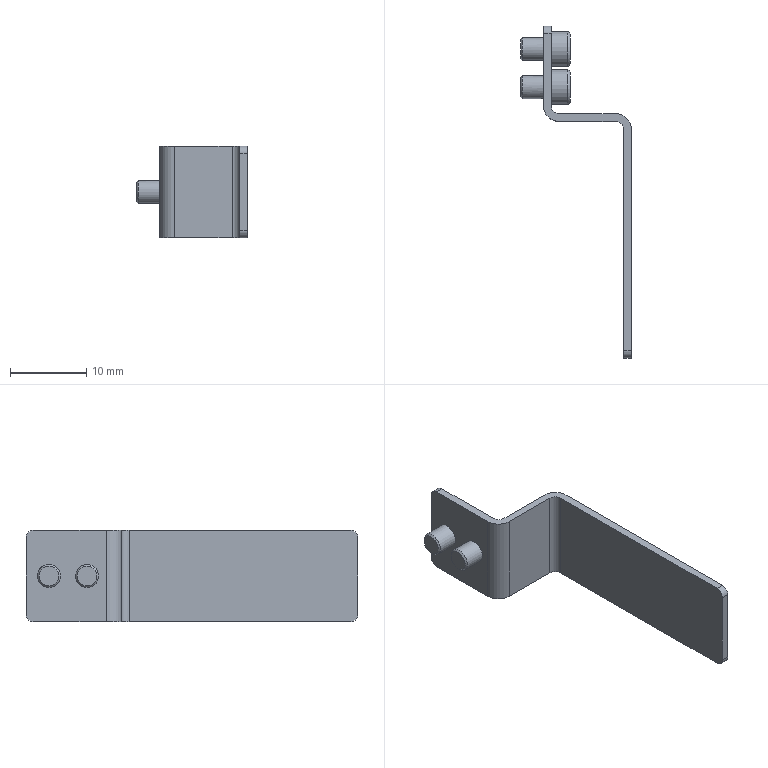Part | STEP file | BODY8_E-RAM6-S-640-ME30-C5 | 1 solid | 44 faces | box 14.5 x 43.5 x 12 mm | volume 744.799 mm3 | plane 28 | cylinder 12 | torus 2 | cone 2 | commonest cylinder face diameters 2 x6 3 x2 4 x2 4.5 x2
STEP:
#1=CARTESIAN_POINT('',(1.,3.,5.));
#2=VERTEX_POINT('',#1);
#3=CARTESIAN_POINT('',(1.,3.,-5.));
#4=VERTEX_POINT('',#3);
#5=CARTESIAN_POINT('',(1.,3.,6.));
#6=DIRECTION('',(0.,0.,-1.));
#7=VECTOR('',#6,1000.);
#8=LINE('',#5,#7);
#9=EDGE_CURVE('',#2,#4,#8,.T.);
#10=ORIENTED_EDGE('',*,*,#9,.T.);
#11=CARTESIAN_POINT('',(0.,3.,-5.));
#12=VERTEX_POINT('',#11);
#13=CARTESIAN_POINT('',(0.,3.,-5.));
#14=DIRECTION('',(-1.,0.,0.));
#15=VECTOR('',#14,1000.);
#16=LINE('',#13,#15);
#17=EDGE_CURVE('',#4,#12,#16,.T.);
#18=ORIENTED_EDGE('',*,*,#17,.T.);
#19=CARTESIAN_POINT('',(0.,3.,5.));
#20=VERTEX_POINT('',#19);
#21=CARTESIAN_POINT('',(0.,3.,6.));
#22=DIRECTION('',(0.,0.,-1.));
#23=VECTOR('',#22,1000.);
#24=LINE('',#21,#23);
#25=EDGE_CURVE('',#20,#12,#24,.T.);
#26=ORIENTED_EDGE('',*,*,#25,.F.);
#27=CARTESIAN_POINT('',(0.,3.,5.));
#28=DIRECTION('',(1.,0.,0.));
#29=VECTOR('',#28,1000.);
#30=LINE('',#27,#29);
#31=EDGE_CURVE('',#20,#2,#30,.T.);
#32=ORIENTED_EDGE('',*,*,#31,.T.);
#33=EDGE_LOOP('',(#10,#18,#26,#32));
#34=FACE_OUTER_BOUND('',#33,.T.);
#35=CARTESIAN_POINT('',(0.,3.,6.));
#36=DIRECTION('',(0.,-1.,0.));
#37=DIRECTION('',(0.,0.,-1.));
#38=AXIS2_PLACEMENT_3D('',#35,#36,#37);
#39=PLANE('',#38);
#40=ADVANCED_FACE('',(#34),#39,.F.);
#41=CARTESIAN_POINT('',(0.,2.,-6.));
#42=VERTEX_POINT('',#41);
#43=CARTESIAN_POINT('',(0.,-7.5,-6.));
#44=VERTEX_POINT('',#43);
#45=CARTESIAN_POINT('',(0.,3.,-6.));
#46=DIRECTION('',(0.,-1.,0.));
#47=VECTOR('',#46,1000.);
#48=LINE('',#45,#47);
#49=EDGE_CURVE('',#42,#44,#48,.T.);
#50=ORIENTED_EDGE('',*,*,#49,.T.);
#51=CARTESIAN_POINT('',(0.,-7.5,6.));
#52=VERTEX_POINT('',#51);
#53=CARTESIAN_POINT('',(0.,-7.5,6.));
#54=DIRECTION('',(0.,0.,1.));
#55=VECTOR('',#54,1000.);
#56=LINE('',#53,#55);
#57=EDGE_CURVE('',#44,#52,#56,.T.);
#58=ORIENTED_EDGE('',*,*,#57,.T.);
#59=CARTESIAN_POINT('',(0.,2.,6.));
#60=VERTEX_POINT('',#59);
#61=CARTESIAN_POINT('',(0.,3.,6.));
#62=DIRECTION('',(0.,-1.,0.));
#63=VECTOR('',#62,1000.);
#64=LINE('',#61,#63);
#65=EDGE_CURVE('',#60,#52,#64,.T.);
#66=ORIENTED_EDGE('',*,*,#65,.F.);
#67=CARTESIAN_POINT('',(0.,2.,5.));
#68=DIRECTION('',(-1.,0.,0.));
#69=DIRECTION('',(0.,0.,-1.));
#70=AXIS2_PLACEMENT_3D('',#67,#68,#69);
#71=CIRCLE('',#70,1.);
#72=EDGE_CURVE('',#60,#20,#71,.T.);
#73=ORIENTED_EDGE('',*,*,#72,.T.);
#74=ORIENTED_EDGE('',*,*,#25,.T.);
#75=CARTESIAN_POINT('',(0.,2.,-5.));
#76=DIRECTION('',(-1.,0.,0.));
#77=DIRECTION('',(0.,0.,-1.));
#78=AXIS2_PLACEMENT_3D('',#75,#76,#77);
#79=CIRCLE('',#78,1.);
#80=EDGE_CURVE('',#12,#42,#79,.T.);
#81=ORIENTED_EDGE('',*,*,#80,.T.);
#82=EDGE_LOOP('',(#50,#58,#66,#73,#74,#81));
#83=FACE_OUTER_BOUND('',#82,.T.);
#84=CARTESIAN_POINT('',(0.,-5.,-1.5));
#85=VERTEX_POINT('',#84);
#86=CARTESIAN_POINT('',(0.,-6.5,0.));
#87=VERTEX_POINT('',#86);
#88=CARTESIAN_POINT('',(0.,-5.,0.));
#89=DIRECTION('',(1.,0.,0.));
#90=DIRECTION('',(0.,0.,-1.));
#91=AXIS2_PLACEMENT_3D('',#88,#89,#90);
#92=CIRCLE('',#91,1.5);
#93=EDGE_CURVE('',#85,#87,#92,.T.);
#94=ORIENTED_EDGE('',*,*,#93,.T.);
#95=CARTESIAN_POINT('',(0.,-5.,0.));
#96=DIRECTION('',(1.,0.,0.));
#97=DIRECTION('',(0.,0.,-1.));
#98=AXIS2_PLACEMENT_3D('',#95,#96,#97);
#99=CIRCLE('',#98,1.5);
#100=EDGE_CURVE('',#87,#85,#99,.T.);
#101=ORIENTED_EDGE('',*,*,#100,.T.);
#102=EDGE_LOOP('',(#94,#101));
#103=FACE_BOUND('',#102,.T.);
#104=CARTESIAN_POINT('',(0.,0.,-1.5));
#105=VERTEX_POINT('',#104);
#106=CARTESIAN_POINT('',(0.,-1.5,0.));
#107=VERTEX_POINT('',#106);
#108=CARTESIAN_POINT('',(0.,0.,0.));
#109=DIRECTION('',(1.,0.,0.));
#110=DIRECTION('',(0.,0.,-1.));
#111=AXIS2_PLACEMENT_3D('',#108,#109,#110);
#112=CIRCLE('',#111,1.5);
#113=EDGE_CURVE('',#105,#107,#112,.T.);
#114=ORIENTED_EDGE('',*,*,#113,.T.);
#115=CARTESIAN_POINT('',(0.,0.,0.));
#116=DIRECTION('',(1.,0.,0.));
#117=DIRECTION('',(0.,0.,-1.));
#118=AXIS2_PLACEMENT_3D('',#115,#116,#117);
#119=CIRCLE('',#118,1.5);
#120=EDGE_CURVE('',#107,#105,#119,.T.);
#121=ORIENTED_EDGE('',*,*,#120,.T.);
#122=EDGE_LOOP('',(#114,#121));
#123=FACE_BOUND('',#122,.T.);
#124=CARTESIAN_POINT('',(0.,3.,6.));
#125=DIRECTION('',(1.,0.,0.));
#126=DIRECTION('',(0.,0.,-1.));
#127=AXIS2_PLACEMENT_3D('',#124,#125,#126);
#128=PLANE('',#127);
#129=ADVANCED_FACE('',(#83,#103,#123),#128,.F.);
#130=CARTESIAN_POINT('',(2.,-9.5,6.));
#131=VERTEX_POINT('',#130);
#132=CARTESIAN_POINT('',(9.5,-9.5,6.));
#133=VERTEX_POINT('',#132);
#134=CARTESIAN_POINT('',(0.,-9.5,6.));
#135=DIRECTION('',(1.,0.,0.));
#136=VECTOR('',#135,1000.);
#137=LINE('',#134,#136);
#138=EDGE_CURVE('',#131,#133,#137,.T.);
#139=ORIENTED_EDGE('',*,*,#138,.F.);
#140=CARTESIAN_POINT('',(2.,-9.5,-6.));
#141=VERTEX_POINT('',#140);
#142=CARTESIAN_POINT('',(2.,-9.5,6.));
#143=DIRECTION('',(0.,0.,-1.));
#144=VECTOR('',#143,1000.);
#145=LINE('',#142,#144);
#146=EDGE_CURVE('',#131,#141,#145,.T.);
#147=ORIENTED_EDGE('',*,*,#146,.T.);
#148=CARTESIAN_POINT('',(9.5,-9.5,-6.));
#149=VERTEX_POINT('',#148);
#150=CARTESIAN_POINT('',(0.,-9.5,-6.));
#151=DIRECTION('',(1.,0.,0.));
#152=VECTOR('',#151,1000.);
#153=LINE('',#150,#152);
#154=EDGE_CURVE('',#141,#149,#153,.T.);
#155=ORIENTED_EDGE('',*,*,#154,.T.);
#156=CARTESIAN_POINT('',(9.5,-9.5,6.));
#157=DIRECTION('',(0.,0.,1.));
#158=VECTOR('',#157,1000.);
#159=LINE('',#156,#158);
#160=EDGE_CURVE('',#149,#133,#159,.T.);
#161=ORIENTED_EDGE('',*,*,#160,.T.);
#162=EDGE_LOOP('',(#139,#147,#155,#161));
#163=FACE_OUTER_BOUND('',#162,.T.);
#164=CARTESIAN_POINT('',(0.,-9.5,6.));
#165=DIRECTION('',(0.,1.,0.));
#166=DIRECTION('',(0.,0.,1.));
#167=AXIS2_PLACEMENT_3D('',#164,#165,#166);
#168=PLANE('',#167);
#169=ADVANCED_FACE('',(#163),#168,.F.);
#170=CARTESIAN_POINT('',(10.5,-10.5,6.));
#171=VERTEX_POINT('',#170);
#172=CARTESIAN_POINT('',(10.5,-39.5,6.));
#173=VERTEX_POINT('',#172);
#174=CARTESIAN_POINT('',(10.5,-9.5,6.));
#175=DIRECTION('',(0.,-1.,0.));
#176=VECTOR('',#175,1000.);
#177=LINE('',#174,#176);
#178=EDGE_CURVE('',#171,#173,#177,.T.);
#179=ORIENTED_EDGE('',*,*,#178,.F.);
#180=CARTESIAN_POINT('',(10.5,-10.5,-6.));
#181=VERTEX_POINT('',#180);
#182=CARTESIAN_POINT('',(10.5,-10.5,-6.));
#183=DIRECTION('',(0.,0.,-1.));
#184=VECTOR('',#183,1000.);
#185=LINE('',#182,#184);
#186=EDGE_CURVE('',#171,#181,#185,.T.);
#187=ORIENTED_EDGE('',*,*,#186,.T.);
#188=CARTESIAN_POINT('',(10.5,-39.5,-6.));
#189=VERTEX_POINT('',#188);
#190=CARTESIAN_POINT('',(10.5,-9.5,-6.));
#191=DIRECTION('',(0.,-1.,0.));
#192=VECTOR('',#191,1000.);
#193=LINE('',#190,#192);
#194=EDGE_CURVE('',#181,#189,#193,.T.);
#195=ORIENTED_EDGE('',*,*,#194,.T.);
#196=CARTESIAN_POINT('',(10.5,-40.5,-5.));
#197=VERTEX_POINT('',#196);
#198=CARTESIAN_POINT('',(10.5,-39.5,-5.));
#199=DIRECTION('',(-1.,0.,0.));
#200=DIRECTION('',(0.,1.,0.));
#201=AXIS2_PLACEMENT_3D('',#198,#199,#200);
#202=CIRCLE('',#201,1.);
#203=EDGE_CURVE('',#189,#197,#202,.T.);
#204=ORIENTED_EDGE('',*,*,#203,.T.);
#205=CARTESIAN_POINT('',(10.5,-40.5,5.));
#206=VERTEX_POINT('',#205);
#207=CARTESIAN_POINT('',(10.5,-40.5,6.));
#208=DIRECTION('',(0.,0.,-1.));
#209=VECTOR('',#208,1000.);
#210=LINE('',#207,#209);
#211=EDGE_CURVE('',#206,#197,#210,.T.);
#212=ORIENTED_EDGE('',*,*,#211,.F.);
#213=CARTESIAN_POINT('',(10.5,-39.5,5.));
#214=DIRECTION('',(-1.,0.,0.));
#215=DIRECTION('',(0.,1.,0.));
#216=AXIS2_PLACEMENT_3D('',#213,#214,#215);
#217=CIRCLE('',#216,1.);
#218=EDGE_CURVE('',#206,#173,#217,.T.);
#219=ORIENTED_EDGE('',*,*,#218,.T.);
#220=EDGE_LOOP('',(#179,#187,#195,#204,#212,#219));
#221=FACE_OUTER_BOUND('',#220,.T.);
#222=CARTESIAN_POINT('',(10.5,-9.5,6.));
#223=DIRECTION('',(1.,0.,0.));
#224=DIRECTION('',(0.,1.,0.));
#225=AXIS2_PLACEMENT_3D('',#222,#223,#224);
#226=PLANE('',#225);
#227=ADVANCED_FACE('',(#221),#226,.F.);
#228=ORIENTED_EDGE('',*,*,#211,.T.);
#229=CARTESIAN_POINT('',(11.5,-40.5,-5.));
#230=VERTEX_POINT('',#229);
#231=CARTESIAN_POINT('',(11.5,-40.5,-5.));
#232=DIRECTION('',(1.,0.,0.));
#233=VECTOR('',#232,1000.);
#234=LINE('',#231,#233);
#235=EDGE_CURVE('',#197,#230,#234,.T.);
#236=ORIENTED_EDGE('',*,*,#235,.T.);
#237=CARTESIAN_POINT('',(11.5,-40.5,5.));
#238=VERTEX_POINT('',#237);
#239=CARTESIAN_POINT('',(11.5,-40.5,6.));
#240=DIRECTION('',(0.,0.,-1.));
#241=VECTOR('',#240,1000.);
#242=LINE('',#239,#241);
#243=EDGE_CURVE('',#238,#230,#242,.T.);
#244=ORIENTED_EDGE('',*,*,#243,.F.);
#245=CARTESIAN_POINT('',(10.5,-40.5,5.));
#246=DIRECTION('',(-1.,0.,0.));
#247=VECTOR('',#246,1000.);
#248=LINE('',#245,#247);
#249=EDGE_CURVE('',#238,#206,#248,.T.);
#250=ORIENTED_EDGE('',*,*,#249,.T.);
#251=EDGE_LOOP('',(#228,#236,#244,#250));
#252=FACE_OUTER_BOUND('',#251,.T.);
#253=CARTESIAN_POINT('',(10.5,-40.5,6.));
#254=DIRECTION('',(0.,1.,0.));
#255=DIRECTION('',(0.,0.,1.));
#256=AXIS2_PLACEMENT_3D('',#253,#254,#255);
#257=PLANE('',#256);
#258=ADVANCED_FACE('',(#252),#257,.F.);
#259=CARTESIAN_POINT('',(11.5,-39.5,-6.));
#260=VERTEX_POINT('',#259);
#261=CARTESIAN_POINT('',(11.5,-10.5,-6.));
#262=VERTEX_POINT('',#261);
#263=CARTESIAN_POINT('',(11.5,-8.5,-6.));
#264=DIRECTION('',(0.,1.,0.));
#265=VECTOR('',#264,1000.);
#266=LINE('',#263,#265);
#267=EDGE_CURVE('',#260,#262,#266,.T.);
#268=ORIENTED_EDGE('',*,*,#267,.T.);
#269=CARTESIAN_POINT('',(11.5,-10.5,6.));
#270=VERTEX_POINT('',#269);
#271=CARTESIAN_POINT('',(11.5,-10.5,6.));
#272=DIRECTION('',(0.,0.,1.));
#273=VECTOR('',#272,1000.);
#274=LINE('',#271,#273);
#275=EDGE_CURVE('',#262,#270,#274,.T.);
#276=ORIENTED_EDGE('',*,*,#275,.T.);
#277=CARTESIAN_POINT('',(11.5,-39.5,6.));
#278=VERTEX_POINT('',#277);
#279=CARTESIAN_POINT('',(11.5,-8.5,6.));
#280=DIRECTION('',(0.,1.,0.));
#281=VECTOR('',#280,1000.);
#282=LINE('',#279,#281);
#283=EDGE_CURVE('',#278,#270,#282,.T.);
#284=ORIENTED_EDGE('',*,*,#283,.F.);
#285=CARTESIAN_POINT('',(11.5,-39.5,5.));
#286=DIRECTION('',(1.,0.,0.));
#287=DIRECTION('',(0.,-1.,0.));
#288=AXIS2_PLACEMENT_3D('',#285,#286,#287);
#289=CIRCLE('',#288,1.);
#290=EDGE_CURVE('',#278,#238,#289,.T.);
#291=ORIENTED_EDGE('',*,*,#290,.T.);
#292=ORIENTED_EDGE('',*,*,#243,.T.);
#293=CARTESIAN_POINT('',(11.5,-39.5,-5.));
#294=DIRECTION('',(1.,0.,0.));
#295=DIRECTION('',(0.,-1.,0.));
#296=AXIS2_PLACEMENT_3D('',#293,#294,#295);
#297=CIRCLE('',#296,1.);
#298=EDGE_CURVE('',#230,#260,#297,.T.);
#299=ORIENTED_EDGE('',*,*,#298,.T.);
#300=EDGE_LOOP('',(#268,#276,#284,#291,#292,#299));
#301=FACE_OUTER_BOUND('',#300,.T.);
#302=CARTESIAN_POINT('',(11.5,-8.5,6.));
#303=DIRECTION('',(-1.,0.,0.));
#304=DIRECTION('',(0.,-1.,0.));
#305=AXIS2_PLACEMENT_3D('',#302,#303,#304);
#306=PLANE('',#305);
#307=ADVANCED_FACE('',(#301),#306,.F.);
#308=CARTESIAN_POINT('',(9.5,-8.5,6.));
#309=VERTEX_POINT('',#308);
#310=CARTESIAN_POINT('',(2.,-8.5,6.));
#311=VERTEX_POINT('',#310);
#312=CARTESIAN_POINT('',(1.,-8.5,6.));
#313=DIRECTION('',(-1.,0.,0.));
#314=VECTOR('',#313,1000.);
#315=LINE('',#312,#314);
#316=EDGE_CURVE('',#309,#311,#315,.T.);
#317=ORIENTED_EDGE('',*,*,#316,.F.);
#318=CARTESIAN_POINT('',(9.5,-8.5,-6.));
#319=VERTEX_POINT('',#318);
#320=CARTESIAN_POINT('',(9.5,-8.5,6.));
#321=DIRECTION('',(0.,0.,-1.));
#322=VECTOR('',#321,1000.);
#323=LINE('',#320,#322);
#324=EDGE_CURVE('',#309,#319,#323,.T.);
#325=ORIENTED_EDGE('',*,*,#324,.T.);
#326=CARTESIAN_POINT('',(2.,-8.5,-6.));
#327=VERTEX_POINT('',#326);
#328=CARTESIAN_POINT('',(1.,-8.5,-6.));
#329=DIRECTION('',(-1.,0.,0.));
#330=VECTOR('',#329,1000.);
#331=LINE('',#328,#330);
#332=EDGE_CURVE('',#319,#327,#331,.T.);
#333=ORIENTED_EDGE('',*,*,#332,.T.);
#334=CARTESIAN_POINT('',(2.,-8.5,6.));
#335=DIRECTION('',(0.,0.,1.));
#336=VECTOR('',#335,1000.);
#337=LINE('',#334,#336);
#338=EDGE_CURVE('',#327,#311,#337,.T.);
#339=ORIENTED_EDGE('',*,*,#338,.T.);
#340=EDGE_LOOP('',(#317,#325,#333,#339));
#341=FACE_OUTER_BOUND('',#340,.T.);
#342=CARTESIAN_POINT('',(1.,-8.5,6.));
#343=DIRECTION('',(0.,-1.,0.));
#344=DIRECTION('',(0.,0.,-1.));
#345=AXIS2_PLACEMENT_3D('',#342,#343,#344);
#346=PLANE('',#345);
#347=ADVANCED_FACE('',(#341),#346,.F.);
#348=CARTESIAN_POINT('',(1.,-7.5,6.));
#349=VERTEX_POINT('',#348);
#350=CARTESIAN_POINT('',(1.,2.,6.));
#351=VERTEX_POINT('',#350);
#352=CARTESIAN_POINT('',(1.,3.,6.));
#353=DIRECTION('',(0.,1.,0.));
#354=VECTOR('',#353,1000.);
#355=LINE('',#352,#354);
#356=EDGE_CURVE('',#349,#351,#355,.T.);
#357=ORIENTED_EDGE('',*,*,#356,.F.);
#358=CARTESIAN_POINT('',(1.,-7.5,-6.));
#359=VERTEX_POINT('',#358);
#360=CARTESIAN_POINT('',(1.,-7.5,-6.));
#361=DIRECTION('',(0.,0.,-1.));
#362=VECTOR('',#361,1000.);
#363=LINE('',#360,#362);
#364=EDGE_CURVE('',#349,#359,#363,.T.);
#365=ORIENTED_EDGE('',*,*,#364,.T.);
#366=CARTESIAN_POINT('',(1.,2.,-6.));
#367=VERTEX_POINT('',#366);
#368=CARTESIAN_POINT('',(1.,3.,-6.));
#369=DIRECTION('',(0.,1.,0.));
#370=VECTOR('',#369,1000.);
#371=LINE('',#368,#370);
#372=EDGE_CURVE('',#359,#367,#371,.T.);
#373=ORIENTED_EDGE('',*,*,#372,.T.);
#374=CARTESIAN_POINT('',(1.,2.,-5.));
#375=DIRECTION('',(1.,0.,0.));
#376=DIRECTION('',(0.,-1.,0.));
#377=AXIS2_PLACEMENT_3D('',#374,#375,#376);
#378=CIRCLE('',#377,1.);
#379=EDGE_CURVE('',#367,#4,#378,.T.);
#380=ORIENTED_EDGE('',*,*,#379,.T.);
#381=ORIENTED_EDGE('',*,*,#9,.F.);
#382=CARTESIAN_POINT('',(1.,2.,5.));
#383=DIRECTION('',(1.,0.,0.));
#384=DIRECTION('',(0.,-1.,0.));
#385=AXIS2_PLACEMENT_3D('',#382,#383,#384);
#386=CIRCLE('',#385,1.);
#387=EDGE_CURVE('',#2,#351,#386,.T.);
#388=ORIENTED_EDGE('',*,*,#387,.T.);
#389=EDGE_LOOP('',(#357,#365,#373,#380,#381,#388));
#390=FACE_OUTER_BOUND('',#389,.T.);
#391=CARTESIAN_POINT('',(1.,-7.25,0.));
#392=VERTEX_POINT('',#391);
#393=CARTESIAN_POINT('',(1.,-2.75,0.));
#394=VERTEX_POINT('',#393);
#395=CARTESIAN_POINT('',(1.,-5.,0.));
#396=DIRECTION('',(1.,0.,0.));
#397=DIRECTION('',(0.,-1.,0.));
#398=AXIS2_PLACEMENT_3D('',#395,#396,#397);
#399=CIRCLE('',#398,2.25);
#400=EDGE_CURVE('',#392,#394,#399,.T.);
#401=ORIENTED_EDGE('',*,*,#400,.F.);
#402=CARTESIAN_POINT('',(1.,-5.,0.));
#403=DIRECTION('',(1.,0.,0.));
#404=DIRECTION('',(0.,-1.,0.));
#405=AXIS2_PLACEMENT_3D('',#402,#403,#404);
#406=CIRCLE('',#405,2.25);
#407=EDGE_CURVE('',#394,#392,#406,.T.);
#408=ORIENTED_EDGE('',*,*,#407,.F.);
#409=EDGE_LOOP('',(#401,#408));
#410=FACE_BOUND('',#409,.T.);
#411=CARTESIAN_POINT('',(1.,-2.25,0.));
#412=VERTEX_POINT('',#411);
#413=CARTESIAN_POINT('',(1.,2.25,0.));
#414=VERTEX_POINT('',#413);
#415=CARTESIAN_POINT('',(1.,0.,0.));
#416=DIRECTION('',(1.,0.,0.));
#417=DIRECTION('',(0.,-1.,0.));
#418=AXIS2_PLACEMENT_3D('',#415,#416,#417);
#419=CIRCLE('',#418,2.25);
#420=EDGE_CURVE('',#412,#414,#419,.T.);
#421=ORIENTED_EDGE('',*,*,#420,.F.);
#422=CARTESIAN_POINT('',(1.,0.,0.));
#423=DIRECTION('',(1.,0.,0.));
#424=DIRECTION('',(0.,-1.,0.));
#425=AXIS2_PLACEMENT_3D('',#422,#423,#424);
#426=CIRCLE('',#425,2.25);
#427=EDGE_CURVE('',#414,#412,#426,.T.);
#428=ORIENTED_EDGE('',*,*,#427,.F.);
#429=EDGE_LOOP('',(#421,#428));
#430=FACE_BOUND('',#429,.T.);
#431=CARTESIAN_POINT('',(1.,3.,6.));
#432=DIRECTION('',(-1.,0.,0.));
#433=DIRECTION('',(0.,-1.,0.));
#434=AXIS2_PLACEMENT_3D('',#431,#432,#433);
#435=PLANE('',#434);
#436=ADVANCED_FACE('',(#390,#410,#430),#435,.F.);
#437=ORIENTED_EDGE('',*,*,#283,.T.);
#438=CARTESIAN_POINT('',(9.5,-10.5,6.));
#439=DIRECTION('',(0.,0.,1.));
#440=DIRECTION('',(-1.,0.,0.));
#441=AXIS2_PLACEMENT_3D('',#438,#439,#440);
#442=CIRCLE('',#441,2.);
#443=EDGE_CURVE('',#270,#309,#442,.T.);
#444=ORIENTED_EDGE('',*,*,#443,.T.);
#445=ORIENTED_EDGE('',*,*,#316,.T.);
#446=CARTESIAN_POINT('',(2.,-7.5,6.));
#447=DIRECTION('',(0.,0.,-1.));
#448=DIRECTION('',(-1.,0.,0.));
#449=AXIS2_PLACEMENT_3D('',#446,#447,#448);
#450=CIRCLE('',#449,1.);
#451=EDGE_CURVE('',#311,#349,#450,.T.);
#452=ORIENTED_EDGE('',*,*,#451,.T.);
#453=ORIENTED_EDGE('',*,*,#356,.T.);
#454=CARTESIAN_POINT('',(0.,2.,6.));
#455=DIRECTION('',(-1.,0.,0.));
#456=VECTOR('',#455,1000.);
#457=LINE('',#454,#456);
#458=EDGE_CURVE('',#351,#60,#457,.T.);
#459=ORIENTED_EDGE('',*,*,#458,.T.);
#460=ORIENTED_EDGE('',*,*,#65,.T.);
#461=CARTESIAN_POINT('',(2.,-7.5,6.));
#462=DIRECTION('',(0.,0.,1.));
#463=DIRECTION('',(-1.,0.,0.));
#464=AXIS2_PLACEMENT_3D('',#461,#462,#463);
#465=CIRCLE('',#464,2.);
#466=EDGE_CURVE('',#52,#131,#465,.T.);
#467=ORIENTED_EDGE('',*,*,#466,.T.);
#468=ORIENTED_EDGE('',*,*,#138,.T.);
#469=CARTESIAN_POINT('',(9.5,-10.5,6.));
#470=DIRECTION('',(0.,0.,-1.));
#471=DIRECTION('',(-1.,0.,0.));
#472=AXIS2_PLACEMENT_3D('',#469,#470,#471);
#473=CIRCLE('',#472,1.);
#474=EDGE_CURVE('',#133,#171,#473,.T.);
#475=ORIENTED_EDGE('',*,*,#474,.T.);
#476=ORIENTED_EDGE('',*,*,#178,.T.);
#477=CARTESIAN_POINT('',(0.,-39.5,6.));
#478=DIRECTION('',(1.,0.,0.));
#479=VECTOR('',#478,1000.);
#480=LINE('',#477,#479);
#481=EDGE_CURVE('',#173,#278,#480,.T.);
#482=ORIENTED_EDGE('',*,*,#481,.T.);
#483=EDGE_LOOP('',(#437,#444,#445,#452,#453,#459,#460,#467,#468,#475,#476,#482));
#484=FACE_OUTER_BOUND('',#483,.T.);
#485=CARTESIAN_POINT('',(0.,0.,6.));
#486=DIRECTION('',(0.,0.,-1.));
#487=DIRECTION('',(-1.,0.,0.));
#488=AXIS2_PLACEMENT_3D('',#485,#486,#487);
#489=PLANE('',#488);
#490=ADVANCED_FACE('',(#484),#489,.F.);
#491=ORIENTED_EDGE('',*,*,#332,.F.);
#492=CARTESIAN_POINT('',(9.5,-10.5,-6.));
#493=DIRECTION('',(0.,0.,-1.));
#494=DIRECTION('',(-1.,0.,0.));
#495=AXIS2_PLACEMENT_3D('',#492,#493,#494);
#496=CIRCLE('',#495,2.);
#497=EDGE_CURVE('',#319,#262,#496,.T.);
#498=ORIENTED_EDGE('',*,*,#497,.T.);
#499=ORIENTED_EDGE('',*,*,#267,.F.);
#500=CARTESIAN_POINT('',(10.5,-39.5,-6.));
#501=DIRECTION('',(-1.,0.,0.));
#502=VECTOR('',#501,1000.);
#503=LINE('',#500,#502);
#504=EDGE_CURVE('',#260,#189,#503,.T.);
#505=ORIENTED_EDGE('',*,*,#504,.T.);
#506=ORIENTED_EDGE('',*,*,#194,.F.);
#507=CARTESIAN_POINT('',(9.5,-10.5,-6.));
#508=DIRECTION('',(0.,0.,1.));
#509=DIRECTION('',(-1.,0.,0.));
#510=AXIS2_PLACEMENT_3D('',#507,#508,#509);
#511=CIRCLE('',#510,1.);
#512=EDGE_CURVE('',#181,#149,#511,.T.);
#513=ORIENTED_EDGE('',*,*,#512,.T.);
#514=ORIENTED_EDGE('',*,*,#154,.F.);
#515=CARTESIAN_POINT('',(2.,-7.5,-6.));
#516=DIRECTION('',(0.,0.,-1.));
#517=DIRECTION('',(-1.,0.,0.));
#518=AXIS2_PLACEMENT_3D('',#515,#516,#517);
#519=CIRCLE('',#518,2.);
#520=EDGE_CURVE('',#141,#44,#519,.T.);
#521=ORIENTED_EDGE('',*,*,#520,.T.);
#522=ORIENTED_EDGE('',*,*,#49,.F.);
#523=CARTESIAN_POINT('',(1.,2.,-6.));
#524=DIRECTION('',(1.,0.,0.));
#525=VECTOR('',#524,1000.);
#526=LINE('',#523,#525);
#527=EDGE_CURVE('',#42,#367,#526,.T.);
#528=ORIENTED_EDGE('',*,*,#527,.T.);
#529=ORIENTED_EDGE('',*,*,#372,.F.);
#530=CARTESIAN_POINT('',(2.,-7.5,-6.));
#531=DIRECTION('',(0.,0.,1.));
#532=DIRECTION('',(-1.,0.,0.));
#533=AXIS2_PLACEMENT_3D('',#530,#531,#532);
#534=CIRCLE('',#533,1.);
#535=EDGE_CURVE('',#359,#327,#534,.T.);
#536=ORIENTED_EDGE('',*,*,#535,.T.);
#537=EDGE_LOOP('',(#491,#498,#499,#505,#506,#513,#514,#521,#522,#528,#529,#536));
#538=FACE_OUTER_BOUND('',#537,.T.);
#539=CARTESIAN_POINT('',(0.,0.,-6.));
#540=DIRECTION('',(0.,0.,-1.));
#541=DIRECTION('',(-1.,0.,0.));
#542=AXIS2_PLACEMENT_3D('',#539,#540,#541);
#543=PLANE('',#542);
#544=ADVANCED_FACE('',(#538),#543,.T.);
#545=ORIENTED_EDGE('',*,*,#420,.T.);
#546=CARTESIAN_POINT('',(3.12,2.25,0.));
#547=VERTEX_POINT('',#546);
#548=CARTESIAN_POINT('',(3.5,2.25,0.));
#549=DIRECTION('',(1.,0.,0.));
#550=VECTOR('',#549,2.25);
#551=LINE('',#548,#550);
#552=EDGE_CURVE('',#414,#547,#551,.T.);
#553=ORIENTED_EDGE('',*,*,#552,.T.);
#554=CARTESIAN_POINT('',(3.12,-2.25,0.));
#555=VERTEX_POINT('',#554);
#556=CARTESIAN_POINT('',(3.12,0.,0.));
#557=DIRECTION('',(-1.,0.,0.));
#558=DIRECTION('',(0.,1.,0.));
#559=AXIS2_PLACEMENT_3D('',#556,#557,#558);
#560=CIRCLE('',#559,2.25);
#561=EDGE_CURVE('',#547,#555,#560,.T.);
#562=ORIENTED_EDGE('',*,*,#561,.T.);
#563=CARTESIAN_POINT('',(3.12,0.,0.));
#564=DIRECTION('',(-1.,0.,0.));
#565=DIRECTION('',(0.,1.,0.));
#566=AXIS2_PLACEMENT_3D('',#563,#564,#565);
#567=CIRCLE('',#566,2.25);
#568=EDGE_CURVE('',#555,#547,#567,.T.);
#569=ORIENTED_EDGE('',*,*,#568,.T.);
#570=ORIENTED_EDGE('',*,*,#552,.F.);
#571=ORIENTED_EDGE('',*,*,#427,.T.);
#572=EDGE_LOOP('',(#545,#553,#562,#569,#570,#571));
#573=FACE_OUTER_BOUND('',#572,.T.);
#574=CARTESIAN_POINT('',(3.5,0.,0.));
#575=DIRECTION('',(-1.,0.,0.));
#576=DIRECTION('',(0.,-1.,0.));
#577=AXIS2_PLACEMENT_3D('',#574,#575,#576);
#578=CYLINDRICAL_SURFACE('',#577,2.25);
#579=ADVANCED_FACE('',(#573),#578,.T.);
#580=CARTESIAN_POINT('',(3.5,1.87,0.));
#581=VERTEX_POINT('',#580);
#582=CARTESIAN_POINT('',(3.5,-1.87,0.));
#583=VERTEX_POINT('',#582);
#584=CARTESIAN_POINT('',(3.5,0.,0.));
#585=DIRECTION('',(1.,0.,0.));
#586=DIRECTION('',(0.,1.,0.));
#587=AXIS2_PLACEMENT_3D('',#584,#585,#586);
#588=CIRCLE('',#587,1.87);
#589=EDGE_CURVE('',#581,#583,#588,.T.);
#590=ORIENTED_EDGE('',*,*,#589,.T.);
#591=CARTESIAN_POINT('',(3.5,0.,0.));
#592=DIRECTION('',(1.,0.,0.));
#593=DIRECTION('',(0.,1.,0.));
#594=AXIS2_PLACEMENT_3D('',#591,#592,#593);
#595=CIRCLE('',#594,1.87);
#596=EDGE_CURVE('',#583,#581,#595,.T.);
#597=ORIENTED_EDGE('',*,*,#596,.T.);
#598=EDGE_LOOP('',(#590,#597));
#599=FACE_OUTER_BOUND('',#598,.T.);
#600=CARTESIAN_POINT('',(3.5,0.5774,-1.));
#601=VERTEX_POINT('',#600);
#602=CARTESIAN_POINT('',(3.5,1.155,0.));
#603=VERTEX_POINT('',#602);
#604=CARTESIAN_POINT('',(3.5,0.5774,-1.));
#605=DIRECTION('',(0.,0.5,0.866));
#606=VECTOR('',#605,1000.);
#607=LINE('',#604,#606);
#608=EDGE_CURVE('',#601,#603,#607,.T.);
#609=ORIENTED_EDGE('',*,*,#608,.F.);
#610=CARTESIAN_POINT('',(3.5,-0.5774,-1.));
#611=VERTEX_POINT('',#610);
#612=CARTESIAN_POINT('',(3.5,-0.5774,-1.));
#613=DIRECTION('',(0.,1.,0.));
#614=VECTOR('',#613,1000.);
#615=LINE('',#612,#614);
#616=EDGE_CURVE('',#611,#601,#615,.T.);
#617=ORIENTED_EDGE('',*,*,#616,.F.);
#618=CARTESIAN_POINT('',(3.5,-1.155,0.));
#619=VERTEX_POINT('',#618);
#620=CARTESIAN_POINT('',(3.5,-1.155,0.));
#621=DIRECTION('',(0.,0.5,-0.866));
#622=VECTOR('',#621,1000.);
#623=LINE('',#620,#622);
#624=EDGE_CURVE('',#619,#611,#623,.T.);
#625=ORIENTED_EDGE('',*,*,#624,.F.);
#626=CARTESIAN_POINT('',(3.5,-0.5774,1.));
#627=VERTEX_POINT('',#626);
#628=CARTESIAN_POINT('',(3.5,-0.5774,1.));
#629=DIRECTION('',(0.,-0.5,-0.866));
#630=VECTOR('',#629,1000.);
#631=LINE('',#628,#630);
#632=EDGE_CURVE('',#627,#619,#631,.T.);
#633=ORIENTED_EDGE('',*,*,#632,.F.);
#634=CARTESIAN_POINT('',(3.5,0.5774,1.));
#635=VERTEX_POINT('',#634);
#636=CARTESIAN_POINT('',(3.5,0.5774,1.));
#637=DIRECTION('',(0.,-1.,0.));
#638=VECTOR('',#637,1000.);
#639=LINE('',#636,#638);
#640=EDGE_CURVE('',#635,#627,#639,.T.);
#641=ORIENTED_EDGE('',*,*,#640,.F.);
#642=CARTESIAN_POINT('',(3.5,1.155,0.));
#643=DIRECTION('',(0.,-0.5,0.866));
#644=VECTOR('',#643,1000.);
#645=LINE('',#642,#644);
#646=EDGE_CURVE('',#603,#635,#645,.T.);
#647=ORIENTED_EDGE('',*,*,#646,.F.);
#648=EDGE_LOOP('',(#609,#617,#625,#633,#641,#647));
#649=FACE_BOUND('',#648,.T.);
#650=CARTESIAN_POINT('',(3.5,0.,0.));
#651=DIRECTION('',(1.,0.,0.));
#652=DIRECTION('',(0.,1.,0.));
#653=AXIS2_PLACEMENT_3D('',#650,#651,#652);
#654=PLANE('',#653);
#655=ADVANCED_FACE('',(#599,#649),#654,.T.);
#656=ORIENTED_EDGE('',*,*,#400,.T.);
#657=CARTESIAN_POINT('',(3.12,-2.75,0.));
#658=VERTEX_POINT('',#657);
#659=CARTESIAN_POINT('',(3.5,-2.75,0.));
#660=DIRECTION('',(1.,0.,0.));
#661=VECTOR('',#660,2.25);
#662=LINE('',#659,#661);
#663=EDGE_CURVE('',#394,#658,#662,.T.);
#664=ORIENTED_EDGE('',*,*,#663,.T.);
#665=CARTESIAN_POINT('',(3.12,-7.25,0.));
#666=VERTEX_POINT('',#665);
#667=CARTESIAN_POINT('',(3.12,-5.,0.));
#668=DIRECTION('',(-1.,0.,0.));
#669=DIRECTION('',(0.,1.,0.));
#670=AXIS2_PLACEMENT_3D('',#667,#668,#669);
#671=CIRCLE('',#670,2.25);
#672=EDGE_CURVE('',#658,#666,#671,.T.);
#673=ORIENTED_EDGE('',*,*,#672,.T.);
#674=CARTESIAN_POINT('',(3.12,-5.,0.));
#675=DIRECTION('',(-1.,0.,0.));
#676=DIRECTION('',(0.,1.,0.));
#677=AXIS2_PLACEMENT_3D('',#674,#675,#676);
#678=CIRCLE('',#677,2.25);
#679=EDGE_CURVE('',#666,#658,#678,.T.);
#680=ORIENTED_EDGE('',*,*,#679,.T.);
#681=ORIENTED_EDGE('',*,*,#663,.F.);
#682=ORIENTED_EDGE('',*,*,#407,.T.);
#683=EDGE_LOOP('',(#656,#664,#673,#680,#681,#682));
#684=FACE_OUTER_BOUND('',#683,.T.);
#685=CARTESIAN_POINT('',(3.5,-5.,0.));
#686=DIRECTION('',(-1.,0.,0.));
#687=DIRECTION('',(0.,-1.,0.));
#688=AXIS2_PLACEMENT_3D('',#685,#686,#687);
#689=CYLINDRICAL_SURFACE('',#688,2.25);
#690=ADVANCED_FACE('',(#684),#689,.T.);
#691=CARTESIAN_POINT('',(3.5,-3.13,0.));
#692=VERTEX_POINT('',#691);
#693=CARTESIAN_POINT('',(3.5,-6.87,0.));
#694=VERTEX_POINT('',#693);
#695=CARTESIAN_POINT('',(3.5,-5.,0.));
#696=DIRECTION('',(1.,0.,0.));
#697=DIRECTION('',(0.,1.,0.));
#698=AXIS2_PLACEMENT_3D('',#695,#696,#697);
#699=CIRCLE('',#698,1.87);
#700=EDGE_CURVE('',#692,#694,#699,.T.);
#701=ORIENTED_EDGE('',*,*,#700,.T.);
#702=CARTESIAN_POINT('',(3.5,-5.,0.));
#703=DIRECTION('',(1.,0.,0.));
#704=DIRECTION('',(0.,1.,0.));
#705=AXIS2_PLACEMENT_3D('',#702,#703,#704);
#706=CIRCLE('',#705,1.87);
#707=EDGE_CURVE('',#694,#692,#706,.T.);
#708=ORIENTED_EDGE('',*,*,#707,.T.);
#709=EDGE_LOOP('',(#701,#708));
#710=FACE_OUTER_BOUND('',#709,.T.);
#711=CARTESIAN_POINT('',(3.5,-4.423,-1.));
#712=VERTEX_POINT('',#711);
#713=CARTESIAN_POINT('',(3.5,-3.845,0.));
#714=VERTEX_POINT('',#713);
#715=CARTESIAN_POINT('',(3.5,-4.423,-1.));
#716=DIRECTION('',(0.,0.5,0.866));
#717=VECTOR('',#716,1000.);
#718=LINE('',#715,#717);
#719=EDGE_CURVE('',#712,#714,#718,.T.);
#720=ORIENTED_EDGE('',*,*,#719,.F.);
#721=CARTESIAN_POINT('',(3.5,-5.577,-1.));
#722=VERTEX_POINT('',#721);
#723=CARTESIAN_POINT('',(3.5,-5.577,-1.));
#724=DIRECTION('',(0.,1.,0.));
#725=VECTOR('',#724,1000.);
#726=LINE('',#723,#725);
#727=EDGE_CURVE('',#722,#712,#726,.T.);
#728=ORIENTED_EDGE('',*,*,#727,.F.);
#729=CARTESIAN_POINT('',(3.5,-6.155,0.));
#730=VERTEX_POINT('',#729);
#731=CARTESIAN_POINT('',(3.5,-6.155,0.));
#732=DIRECTION('',(0.,0.5,-0.866));
#733=VECTOR('',#732,1000.);
#734=LINE('',#731,#733);
#735=EDGE_CURVE('',#730,#722,#734,.T.);
#736=ORIENTED_EDGE('',*,*,#735,.F.);
#737=CARTESIAN_POINT('',(3.5,-5.577,1.));
#738=VERTEX_POINT('',#737);
#739=CARTESIAN_POINT('',(3.5,-5.577,1.));
#740=DIRECTION('',(0.,-0.5,-0.866));
#741=VECTOR('',#740,1000.);
#742=LINE('',#739,#741);
#743=EDGE_CURVE('',#738,#730,#742,.T.);
#744=ORIENTED_EDGE('',*,*,#743,.F.);
#745=CARTESIAN_POINT('',(3.5,-4.423,1.));
#746=VERTEX_POINT('',#745);
#747=CARTESIAN_POINT('',(3.5,-4.423,1.));
#748=DIRECTION('',(0.,-1.,0.));
#749=VECTOR('',#748,1000.);
#750=LINE('',#747,#749);
#751=EDGE_CURVE('',#746,#738,#750,.T.);
#752=ORIENTED_EDGE('',*,*,#751,.F.);
#753=CARTESIAN_POINT('',(3.5,-3.845,0.));
#754=DIRECTION('',(0.,-0.5,0.866));
#755=VECTOR('',#754,1000.);
#756=LINE('',#753,#755);
#757=EDGE_CURVE('',#714,#746,#756,.T.);
#758=ORIENTED_EDGE('',*,*,#757,.F.);
#759=EDGE_LOOP('',(#720,#728,#736,#744,#752,#758));
#760=FACE_BOUND('',#759,.T.);
#761=CARTESIAN_POINT('',(3.5,-5.,0.));
#762=DIRECTION('',(1.,0.,0.));
#763=DIRECTION('',(0.,1.,0.));
#764=AXIS2_PLACEMENT_3D('',#761,#762,#763);
#765=PLANE('',#764);
#766=ADVANCED_FACE('',(#710,#760),#765,.T.);
#767=ORIENTED_EDGE('',*,*,#608,.T.);
#768=CARTESIAN_POINT('',(2.4,1.155,0.));
#769=VERTEX_POINT('',#768);
#770=CARTESIAN_POINT('',(2.4,1.155,0.));
#771=DIRECTION('',(1.,0.,0.));
#772=VECTOR('',#771,1000.);
#773=LINE('',#770,#772);
#774=EDGE_CURVE('',#769,#603,#773,.T.);
#775=ORIENTED_EDGE('',*,*,#774,.F.);
#776=CARTESIAN_POINT('',(2.4,0.5774,-1.));
#777=VERTEX_POINT('',#776);
#778=CARTESIAN_POINT('',(2.4,0.5774,-1.));
#779=DIRECTION('',(0.,0.5,0.866));
#780=VECTOR('',#779,1000.);
#781=LINE('',#778,#780);
#782=EDGE_CURVE('',#777,#769,#781,.T.);
#783=ORIENTED_EDGE('',*,*,#782,.F.);
#784=CARTESIAN_POINT('',(2.4,0.5774,-1.));
#785=DIRECTION('',(1.,0.,0.));
#786=VECTOR('',#785,1000.);
#787=LINE('',#784,#786);
#788=EDGE_CURVE('',#777,#601,#787,.T.);
#789=ORIENTED_EDGE('',*,*,#788,.T.);
#790=EDGE_LOOP('',(#767,#775,#783,#789));
#791=FACE_OUTER_BOUND('',#790,.T.);
#792=CARTESIAN_POINT('',(2.4,0.5774,-1.));
#793=DIRECTION('',(0.,0.866,-0.5));
#794=DIRECTION('',(0.,0.5,0.866));
#795=AXIS2_PLACEMENT_3D('',#792,#793,#794);
#796=PLANE('',#795);
#797=ADVANCED_FACE('',(#791),#796,.F.);
#798=ORIENTED_EDGE('',*,*,#616,.T.);
#799=ORIENTED_EDGE('',*,*,#788,.F.);
#800=CARTESIAN_POINT('',(2.4,-0.5774,-1.));
#801=VERTEX_POINT('',#800);
#802=CARTESIAN_POINT('',(2.4,-0.5774,-1.));
#803=DIRECTION('',(0.,1.,0.));
#804=VECTOR('',#803,1000.);
#805=LINE('',#802,#804);
#806=EDGE_CURVE('',#801,#777,#805,.T.);
#807=ORIENTED_EDGE('',*,*,#806,.F.);
#808=CARTESIAN_POINT('',(2.4,-0.5774,-1.));
#809=DIRECTION('',(1.,0.,0.));
#810=VECTOR('',#809,1000.);
#811=LINE('',#808,#810);
#812=EDGE_CURVE('',#801,#611,#811,.T.);
#813=ORIENTED_EDGE('',*,*,#812,.T.);
#814=EDGE_LOOP('',(#798,#799,#807,#813));
#815=FACE_OUTER_BOUND('',#814,.T.);
#816=CARTESIAN_POINT('',(2.4,-0.5774,-1.));
#817=DIRECTION('',(0.,0.,-1.));
#818=DIRECTION('',(0.,1.,0.));
#819=AXIS2_PLACEMENT_3D('',#816,#817,#818);
#820=PLANE('',#819);
#821=ADVANCED_FACE('',(#815),#820,.F.);
#822=ORIENTED_EDGE('',*,*,#624,.T.);
#823=ORIENTED_EDGE('',*,*,#812,.F.);
#824=CARTESIAN_POINT('',(2.4,-1.155,0.));
#825=VERTEX_POINT('',#824);
#826=CARTESIAN_POINT('',(2.4,-1.155,0.));
#827=DIRECTION('',(0.,0.5,-0.866));
#828=VECTOR('',#827,1000.);
#829=LINE('',#826,#828);
#830=EDGE_CURVE('',#825,#801,#829,.T.);
#831=ORIENTED_EDGE('',*,*,#830,.F.);
#832=CARTESIAN_POINT('',(2.4,-1.155,0.));
#833=DIRECTION('',(1.,0.,0.));
#834=VECTOR('',#833,1000.);
#835=LINE('',#832,#834);
#836=EDGE_CURVE('',#825,#619,#835,.T.);
#837=ORIENTED_EDGE('',*,*,#836,.T.);
#838=EDGE_LOOP('',(#822,#823,#831,#837));
#839=FACE_OUTER_BOUND('',#838,.T.);
#840=CARTESIAN_POINT('',(2.4,-1.155,0.));
#841=DIRECTION('',(0.,-0.866,-0.5));
#842=DIRECTION('',(0.,0.5,-0.866));
#843=AXIS2_PLACEMENT_3D('',#840,#841,#842);
#844=PLANE('',#843);
#845=ADVANCED_FACE('',(#839),#844,.F.);
#846=ORIENTED_EDGE('',*,*,#632,.T.);
#847=ORIENTED_EDGE('',*,*,#836,.F.);
#848=CARTESIAN_POINT('',(2.4,-0.5774,1.));
#849=VERTEX_POINT('',#848);
#850=CARTESIAN_POINT('',(2.4,-0.5774,1.));
#851=DIRECTION('',(0.,-0.5,-0.866));
#852=VECTOR('',#851,1000.);
#853=LINE('',#850,#852);
#854=EDGE_CURVE('',#849,#825,#853,.T.);
#855=ORIENTED_EDGE('',*,*,#854,.F.);
#856=CARTESIAN_POINT('',(2.4,-0.5774,1.));
#857=DIRECTION('',(1.,0.,0.));
#858=VECTOR('',#857,1000.);
#859=LINE('',#856,#858);
#860=EDGE_CURVE('',#849,#627,#859,.T.);
#861=ORIENTED_EDGE('',*,*,#860,.T.);
#862=EDGE_LOOP('',(#846,#847,#855,#861));
#863=FACE_OUTER_BOUND('',#862,.T.);
#864=CARTESIAN_POINT('',(2.4,-0.5774,1.));
#865=DIRECTION('',(0.,-0.866,0.5));
#866=DIRECTION('',(0.,-0.5,-0.866));
#867=AXIS2_PLACEMENT_3D('',#864,#865,#866);
#868=PLANE('',#867);
#869=ADVANCED_FACE('',(#863),#868,.F.);
#870=ORIENTED_EDGE('',*,*,#640,.T.);
#871=ORIENTED_EDGE('',*,*,#860,.F.);
#872=CARTESIAN_POINT('',(2.4,0.5774,1.));
#873=VERTEX_POINT('',#872);
#874=CARTESIAN_POINT('',(2.4,0.5774,1.));
#875=DIRECTION('',(0.,-1.,0.));
#876=VECTOR('',#875,1000.);
#877=LINE('',#874,#876);
#878=EDGE_CURVE('',#873,#849,#877,.T.);
#879=ORIENTED_EDGE('',*,*,#878,.F.);
#880=CARTESIAN_POINT('',(2.4,0.5774,1.));
#881=DIRECTION('',(1.,0.,0.));
#882=VECTOR('',#881,1000.);
#883=LINE('',#880,#882);
#884=EDGE_CURVE('',#873,#635,#883,.T.);
#885=ORIENTED_EDGE('',*,*,#884,.T.);
#886=EDGE_LOOP('',(#870,#871,#879,#885));
#887=FACE_OUTER_BOUND('',#886,.T.);
#888=CARTESIAN_POINT('',(2.4,0.5774,1.));
#889=DIRECTION('',(0.,0.,1.));
#890=DIRECTION('',(1.,0.,0.));
#891=AXIS2_PLACEMENT_3D('',#888,#889,#890);
#892=PLANE('',#891);
#893=ADVANCED_FACE('',(#887),#892,.F.);
#894=ORIENTED_EDGE('',*,*,#646,.T.);
#895=ORIENTED_EDGE('',*,*,#884,.F.);
#896=CARTESIAN_POINT('',(2.4,1.155,0.));
#897=DIRECTION('',(0.,-0.5,0.866));
#898=VECTOR('',#897,1000.);
#899=LINE('',#896,#898);
#900=EDGE_CURVE('',#769,#873,#899,.T.);
#901=ORIENTED_EDGE('',*,*,#900,.F.);
#902=ORIENTED_EDGE('',*,*,#774,.T.);
#903=EDGE_LOOP('',(#894,#895,#901,#902));
#904=FACE_OUTER_BOUND('',#903,.T.);
#905=CARTESIAN_POINT('',(2.4,1.155,0.));
#906=DIRECTION('',(0.,0.866,0.5));
#907=DIRECTION('',(0.,-0.5,0.866));
#908=AXIS2_PLACEMENT_3D('',#905,#906,#907);
#909=PLANE('',#908);
#910=ADVANCED_FACE('',(#904),#909,.F.);
#911=ORIENTED_EDGE('',*,*,#782,.T.);
#912=ORIENTED_EDGE('',*,*,#900,.T.);
#913=ORIENTED_EDGE('',*,*,#878,.T.);
#914=ORIENTED_EDGE('',*,*,#854,.T.);
#915=ORIENTED_EDGE('',*,*,#830,.T.);
#916=ORIENTED_EDGE('',*,*,#806,.T.);
#917=EDGE_LOOP('',(#911,#912,#913,#914,#915,#916));
#918=FACE_OUTER_BOUND('',#917,.T.);
#919=CARTESIAN_POINT('',(2.4,0.,0.));
#920=DIRECTION('',(1.,0.,0.));
#921=DIRECTION('',(0.,0.,-1.));
#922=AXIS2_PLACEMENT_3D('',#919,#920,#921);
#923=PLANE('',#922);
#924=ADVANCED_FACE('',(#918),#923,.T.);
#925=ORIENTED_EDGE('',*,*,#719,.T.);
#926=CARTESIAN_POINT('',(2.4,-3.845,0.));
#927=VERTEX_POINT('',#926);
#928=CARTESIAN_POINT('',(2.4,-3.845,0.));
#929=DIRECTION('',(1.,0.,0.));
#930=VECTOR('',#929,1000.);
#931=LINE('',#928,#930);
#932=EDGE_CURVE('',#927,#714,#931,.T.);
#933=ORIENTED_EDGE('',*,*,#932,.F.);
#934=CARTESIAN_POINT('',(2.4,-4.423,-1.));
#935=VERTEX_POINT('',#934);
#936=CARTESIAN_POINT('',(2.4,-4.423,-1.));
#937=DIRECTION('',(0.,0.5,0.866));
#938=VECTOR('',#937,1000.);
#939=LINE('',#936,#938);
#940=EDGE_CURVE('',#935,#927,#939,.T.);
#941=ORIENTED_EDGE('',*,*,#940,.F.);
#942=CARTESIAN_POINT('',(2.4,-4.423,-1.));
#943=DIRECTION('',(1.,0.,0.));
#944=VECTOR('',#943,1000.);
#945=LINE('',#942,#944);
#946=EDGE_CURVE('',#935,#712,#945,.T.);
#947=ORIENTED_EDGE('',*,*,#946,.T.);
#948=EDGE_LOOP('',(#925,#933,#941,#947));
#949=FACE_OUTER_BOUND('',#948,.T.);
#950=CARTESIAN_POINT('',(2.4,-4.423,-1.));
#951=DIRECTION('',(0.,0.866,-0.5));
#952=DIRECTION('',(0.,0.5,0.866));
#953=AXIS2_PLACEMENT_3D('',#950,#951,#952);
#954=PLANE('',#953);
#955=ADVANCED_FACE('',(#949),#954,.F.);
#956=ORIENTED_EDGE('',*,*,#727,.T.);
#957=ORIENTED_EDGE('',*,*,#946,.F.);
#958=CARTESIAN_POINT('',(2.4,-5.577,-1.));
#959=VERTEX_POINT('',#958);
#960=CARTESIAN_POINT('',(2.4,-5.577,-1.));
#961=DIRECTION('',(0.,1.,0.));
#962=VECTOR('',#961,1000.);
#963=LINE('',#960,#962);
#964=EDGE_CURVE('',#959,#935,#963,.T.);
#965=ORIENTED_EDGE('',*,*,#964,.F.);
#966=CARTESIAN_POINT('',(2.4,-5.577,-1.));
#967=DIRECTION('',(1.,0.,0.));
#968=VECTOR('',#967,1000.);
#969=LINE('',#966,#968);
#970=EDGE_CURVE('',#959,#722,#969,.T.);
#971=ORIENTED_EDGE('',*,*,#970,.T.);
#972=EDGE_LOOP('',(#956,#957,#965,#971));
#973=FACE_OUTER_BOUND('',#972,.T.);
#974=CARTESIAN_POINT('',(2.4,-5.577,-1.));
#975=DIRECTION('',(0.,0.,-1.));
#976=DIRECTION('',(-1.,0.,0.));
#977=AXIS2_PLACEMENT_3D('',#974,#975,#976);
#978=PLANE('',#977);
#979=ADVANCED_FACE('',(#973),#978,.F.);
#980=ORIENTED_EDGE('',*,*,#735,.T.);
#981=ORIENTED_EDGE('',*,*,#970,.F.);
#982=CARTESIAN_POINT('',(2.4,-6.155,0.));
#983=VERTEX_POINT('',#982);
#984=CARTESIAN_POINT('',(2.4,-6.155,0.));
#985=DIRECTION('',(0.,0.5,-0.866));
#986=VECTOR('',#985,1000.);
#987=LINE('',#984,#986);
#988=EDGE_CURVE('',#983,#959,#987,.T.);
#989=ORIENTED_EDGE('',*,*,#988,.F.);
#990=CARTESIAN_POINT('',(2.4,-6.155,0.));
#991=DIRECTION('',(1.,0.,0.));
#992=VECTOR('',#991,1000.);
#993=LINE('',#990,#992);
#994=EDGE_CURVE('',#983,#730,#993,.T.);
#995=ORIENTED_EDGE('',*,*,#994,.T.);
#996=EDGE_LOOP('',(#980,#981,#989,#995));
#997=FACE_OUTER_BOUND('',#996,.T.);
#998=CARTESIAN_POINT('',(2.4,-6.155,0.));
#999=DIRECTION('',(0.,-0.866,-0.5));
#1000=DIRECTION('',(0.,0.5,-0.866));
#1001=AXIS2_PLACEMENT_3D('',#998,#999,#1000);
#1002=PLANE('',#1001);
#1003=ADVANCED_FACE('',(#997),#1002,.F.);
#1004=ORIENTED_EDGE('',*,*,#743,.T.);
#1005=ORIENTED_EDGE('',*,*,#994,.F.);
#1006=CARTESIAN_POINT('',(2.4,-5.577,1.));
#1007=VERTEX_POINT('',#1006);
#1008=CARTESIAN_POINT('',(2.4,-5.577,1.));
#1009=DIRECTION('',(0.,-0.5,-0.866));
#1010=VECTOR('',#1009,1000.);
#1011=LINE('',#1008,#1010);
#1012=EDGE_CURVE('',#1007,#983,#1011,.T.);
#1013=ORIENTED_EDGE('',*,*,#1012,.F.);
#1014=CARTESIAN_POINT('',(2.4,-5.577,1.));
#1015=DIRECTION('',(1.,0.,0.));
#1016=VECTOR('',#1015,1000.);
#1017=LINE('',#1014,#1016);
#1018=EDGE_CURVE('',#1007,#738,#1017,.T.);
#1019=ORIENTED_EDGE('',*,*,#1018,.T.);
#1020=EDGE_LOOP('',(#1004,#1005,#1013,#1019));
#1021=FACE_OUTER_BOUND('',#1020,.T.);
#1022=CARTESIAN_POINT('',(2.4,-5.577,1.));
#1023=DIRECTION('',(0.,-0.866,0.5));
#1024=DIRECTION('',(0.,-0.5,-0.866));
#1025=AXIS2_PLACEMENT_3D('',#1022,#1023,#1024);
#1026=PLANE('',#1025);
#1027=ADVANCED_FACE('',(#1021),#1026,.F.);
#1028=ORIENTED_EDGE('',*,*,#751,.T.);
#1029=ORIENTED_EDGE('',*,*,#1018,.F.);
#1030=CARTESIAN_POINT('',(2.4,-4.423,1.));
#1031=VERTEX_POINT('',#1030);
#1032=CARTESIAN_POINT('',(2.4,-4.423,1.));
#1033=DIRECTION('',(0.,-1.,0.));
#1034=VECTOR('',#1033,1000.);
#1035=LINE('',#1032,#1034);
#1036=EDGE_CURVE('',#1031,#1007,#1035,.T.);
#1037=ORIENTED_EDGE('',*,*,#1036,.F.);
#1038=CARTESIAN_POINT('',(2.4,-4.423,1.));
#1039=DIRECTION('',(1.,0.,0.));
#1040=VECTOR('',#1039,1000.);
#1041=LINE('',#1038,#1040);
#1042=EDGE_CURVE('',#1031,#746,#1041,.T.);
#1043=ORIENTED_EDGE('',*,*,#1042,.T.);
#1044=EDGE_LOOP('',(#1028,#1029,#1037,#1043));
#1045=FACE_OUTER_BOUND('',#1044,.T.);
#1046=CARTESIAN_POINT('',(2.4,-4.423,1.));
#1047=DIRECTION('',(0.,0.,1.));
#1048=DIRECTION('',(0.,-1.,0.));
#1049=AXIS2_PLACEMENT_3D('',#1046,#1047,#1048);
#1050=PLANE('',#1049);
#1051=ADVANCED_FACE('',(#1045),#1050,.F.);
#1052=ORIENTED_EDGE('',*,*,#757,.T.);
#1053=ORIENTED_EDGE('',*,*,#1042,.F.);
#1054=CARTESIAN_POINT('',(2.4,-3.845,0.));
#1055=DIRECTION('',(0.,-0.5,0.866));
#1056=VECTOR('',#1055,1000.);
#1057=LINE('',#1054,#1056);
#1058=EDGE_CURVE('',#927,#1031,#1057,.T.);
#1059=ORIENTED_EDGE('',*,*,#1058,.F.);
#1060=ORIENTED_EDGE('',*,*,#932,.T.);
#1061=EDGE_LOOP('',(#1052,#1053,#1059,#1060));
#1062=FACE_OUTER_BOUND('',#1061,.T.);
#1063=CARTESIAN_POINT('',(2.4,-3.845,0.));
#1064=DIRECTION('',(0.,0.866,0.5));
#1065=DIRECTION('',(0.,-0.5,0.866));
#1066=AXIS2_PLACEMENT_3D('',#1063,#1064,#1065);
#1067=PLANE('',#1066);
#1068=ADVANCED_FACE('',(#1062),#1067,.F.);
#1069=ORIENTED_EDGE('',*,*,#940,.T.);
#1070=ORIENTED_EDGE('',*,*,#1058,.T.);
#1071=ORIENTED_EDGE('',*,*,#1036,.T.);
#1072=ORIENTED_EDGE('',*,*,#1012,.T.);
#1073=ORIENTED_EDGE('',*,*,#988,.T.);
#1074=ORIENTED_EDGE('',*,*,#964,.T.);
#1075=EDGE_LOOP('',(#1069,#1070,#1071,#1072,#1073,#1074));
#1076=FACE_OUTER_BOUND('',#1075,.T.);
#1077=CARTESIAN_POINT('',(2.4,0.,0.));
#1078=DIRECTION('',(1.,0.,0.));
#1079=DIRECTION('',(0.,0.,-1.));
#1080=AXIS2_PLACEMENT_3D('',#1077,#1078,#1079);
#1081=PLANE('',#1080);
#1082=ADVANCED_FACE('',(#1076),#1081,.T.);
#1083=ORIENTED_EDGE('',*,*,#113,.F.);
#1084=ORIENTED_EDGE('',*,*,#120,.F.);
#1085=CARTESIAN_POINT('',(-2.8,-1.5,0.));
#1086=VERTEX_POINT('',#1085);
#1087=CARTESIAN_POINT('',(-3.,-1.5,0.));
#1088=DIRECTION('',(-1.,0.,0.));
#1089=VECTOR('',#1088,1.5);
#1090=LINE('',#1087,#1089);
#1091=EDGE_CURVE('',#107,#1086,#1090,.T.);
#1092=ORIENTED_EDGE('',*,*,#1091,.T.);
#1093=CARTESIAN_POINT('',(-2.8,1.5,0.));
#1094=VERTEX_POINT('',#1093);
#1095=CARTESIAN_POINT('',(-2.8,0.,0.));
#1096=DIRECTION('',(1.,0.,0.));
#1097=DIRECTION('',(0.,1.,0.));
#1098=AXIS2_PLACEMENT_3D('',#1095,#1096,#1097);
#1099=CIRCLE('',#1098,1.5);
#1100=EDGE_CURVE('',#1086,#1094,#1099,.T.);
#1101=ORIENTED_EDGE('',*,*,#1100,.T.);
#1102=CARTESIAN_POINT('',(-2.8,0.,0.));
#1103=DIRECTION('',(1.,0.,0.));
#1104=DIRECTION('',(0.,1.,0.));
#1105=AXIS2_PLACEMENT_3D('',#1102,#1103,#1104);
#1106=CIRCLE('',#1105,1.5);
#1107=EDGE_CURVE('',#1094,#1086,#1106,.T.);
#1108=ORIENTED_EDGE('',*,*,#1107,.T.);
#1109=ORIENTED_EDGE('',*,*,#1091,.F.);
#1110=EDGE_LOOP('',(#1083,#1084,#1092,#1101,#1108,#1109));
#1111=FACE_OUTER_BOUND('',#1110,.T.);
#1112=CARTESIAN_POINT('',(-3.,0.,0.));
#1113=DIRECTION('',(1.,0.,0.));
#1114=DIRECTION('',(0.,1.,0.));
#1115=AXIS2_PLACEMENT_3D('',#1112,#1113,#1114);
#1116=CYLINDRICAL_SURFACE('',#1115,1.5);
#1117=ADVANCED_FACE('',(#1111),#1116,.T.);
#1118=CARTESIAN_POINT('',(-3.,1.3,0.));
#1119=VERTEX_POINT('',#1118);
#1120=CARTESIAN_POINT('',(-3.,-1.3,0.));
#1121=VERTEX_POINT('',#1120);
#1122=CARTESIAN_POINT('',(-3.,0.,0.));
#1123=DIRECTION('',(-1.,0.,0.));
#1124=DIRECTION('',(0.,1.,0.));
#1125=AXIS2_PLACEMENT_3D('',#1122,#1123,#1124);
#1126=CIRCLE('',#1125,1.3);
#1127=EDGE_CURVE('',#1119,#1121,#1126,.T.);
#1128=ORIENTED_EDGE('',*,*,#1127,.T.);
#1129=CARTESIAN_POINT('',(-3.,0.,0.));
#1130=DIRECTION('',(-1.,0.,0.));
#1131=DIRECTION('',(0.,1.,0.));
#1132=AXIS2_PLACEMENT_3D('',#1129,#1130,#1131);
#1133=CIRCLE('',#1132,1.3);
#1134=EDGE_CURVE('',#1121,#1119,#1133,.T.);
#1135=ORIENTED_EDGE('',*,*,#1134,.T.);
#1136=EDGE_LOOP('',(#1128,#1135));
#1137=FACE_OUTER_BOUND('',#1136,.T.);
#1138=CARTESIAN_POINT('',(-3.,0.,0.));
#1139=DIRECTION('',(1.,0.,0.));
#1140=DIRECTION('',(0.,1.,0.));
#1141=AXIS2_PLACEMENT_3D('',#1138,#1139,#1140);
#1142=PLANE('',#1141);
#1143=ADVANCED_FACE('',(#1137),#1142,.F.);
#1144=ORIENTED_EDGE('',*,*,#93,.F.);
#1145=ORIENTED_EDGE('',*,*,#100,.F.);
#1146=CARTESIAN_POINT('',(-2.8,-6.5,0.));
#1147=VERTEX_POINT('',#1146);
#1148=CARTESIAN_POINT('',(-3.,-6.5,0.));
#1149=DIRECTION('',(-1.,0.,0.));
#1150=VECTOR('',#1149,1.5);
#1151=LINE('',#1148,#1150);
#1152=EDGE_CURVE('',#87,#1147,#1151,.T.);
#1153=ORIENTED_EDGE('',*,*,#1152,.T.);
#1154=CARTESIAN_POINT('',(-2.8,-5.,-1.5));
#1155=VERTEX_POINT('',#1154);
#1156=CARTESIAN_POINT('',(-2.8,-5.,0.));
#1157=DIRECTION('',(1.,0.,0.));
#1158=DIRECTION('',(0.,0.,-1.));
#1159=AXIS2_PLACEMENT_3D('',#1156,#1157,#1158);
#1160=CIRCLE('',#1159,1.5);
#1161=EDGE_CURVE('',#1147,#1155,#1160,.T.);
#1162=ORIENTED_EDGE('',*,*,#1161,.T.);
#1163=CARTESIAN_POINT('',(-2.8,-5.,1.5));
#1164=VERTEX_POINT('',#1163);
#1165=CARTESIAN_POINT('',(-2.8,-5.,0.));
#1166=DIRECTION('',(1.,0.,0.));
#1167=DIRECTION('',(0.,0.,-1.));
#1168=AXIS2_PLACEMENT_3D('',#1165,#1166,#1167);
#1169=CIRCLE('',#1168,1.5);
#1170=EDGE_CURVE('',#1155,#1164,#1169,.T.);
#1171=ORIENTED_EDGE('',*,*,#1170,.T.);
#1172=CARTESIAN_POINT('',(-2.8,-5.,0.));
#1173=DIRECTION('',(1.,0.,0.));
#1174=DIRECTION('',(0.,0.,-1.));
#1175=AXIS2_PLACEMENT_3D('',#1172,#1173,#1174);
#1176=CIRCLE('',#1175,1.5);
#1177=EDGE_CURVE('',#1164,#1147,#1176,.T.);
#1178=ORIENTED_EDGE('',*,*,#1177,.T.);
#1179=ORIENTED_EDGE('',*,*,#1152,.F.);
#1180=EDGE_LOOP('',(#1144,#1145,#1153,#1162,#1171,#1178,#1179));
#1181=FACE_OUTER_BOUND('',#1180,.T.);
#1182=CARTESIAN_POINT('',(-3.,-5.,0.));
#1183=DIRECTION('',(1.,0.,0.));
#1184=DIRECTION('',(0.,1.,0.));
#1185=AXIS2_PLACEMENT_3D('',#1182,#1183,#1184);
#1186=CYLINDRICAL_SURFACE('',#1185,1.5);
#1187=ADVANCED_FACE('',(#1181),#1186,.T.);
#1188=CARTESIAN_POINT('',(-3.,-3.7,0.));
#1189=VERTEX_POINT('',#1188);
#1190=CARTESIAN_POINT('',(-3.,-5.,1.3));
#1191=VERTEX_POINT('',#1190);
#1192=CARTESIAN_POINT('',(-3.,-5.,0.));
#1193=DIRECTION('',(-1.,0.,0.));
#1194=DIRECTION('',(0.,1.,0.));
#1195=AXIS2_PLACEMENT_3D('',#1192,#1193,#1194);
#1196=CIRCLE('',#1195,1.3);
#1197=EDGE_CURVE('',#1189,#1191,#1196,.T.);
#1198=ORIENTED_EDGE('',*,*,#1197,.T.);
#1199=CARTESIAN_POINT('',(-3.,-5.,0.));
#1200=DIRECTION('',(-1.,0.,0.));
#1201=DIRECTION('',(0.,1.,0.));
#1202=AXIS2_PLACEMENT_3D('',#1199,#1200,#1201);
#1203=CIRCLE('',#1202,1.3);
#1204=EDGE_CURVE('',#1191,#1189,#1203,.T.);
#1205=ORIENTED_EDGE('',*,*,#1204,.T.);
#1206=EDGE_LOOP('',(#1198,#1205));
#1207=FACE_OUTER_BOUND('',#1206,.T.);
#1208=CARTESIAN_POINT('',(-3.,-5.,0.));
#1209=DIRECTION('',(1.,0.,0.));
#1210=DIRECTION('',(0.,1.,0.));
#1211=AXIS2_PLACEMENT_3D('',#1208,#1209,#1210);
#1212=PLANE('',#1211);
#1213=ADVANCED_FACE('',(#1207),#1212,.F.);
#1214=ORIENTED_EDGE('',*,*,#700,.F.);
#1215=ORIENTED_EDGE('',*,*,#707,.F.);
#1216=CARTESIAN_POINT('',(3.12,-6.87,0.));
#1217=DIRECTION('',(0.,0.,-1.));
#1218=DIRECTION('',(0.,-1.,0.));
#1219=AXIS2_PLACEMENT_3D('',#1216,#1217,#1218);
#1220=CIRCLE('',#1219,0.38);
#1221=EDGE_CURVE('',#694,#666,#1220,.T.);
#1222=ORIENTED_EDGE('',*,*,#1221,.T.);
#1223=ORIENTED_EDGE('',*,*,#672,.F.);
#1224=ORIENTED_EDGE('',*,*,#679,.F.);
#1225=ORIENTED_EDGE('',*,*,#1221,.F.);
#1226=EDGE_LOOP('',(#1214,#1215,#1222,#1223,#1224,#1225));
#1227=FACE_OUTER_BOUND('',#1226,.T.);
#1228=CARTESIAN_POINT('',(3.12,-5.,0.));
#1229=DIRECTION('',(1.,0.,0.));
#1230=DIRECTION('',(0.,1.,0.));
#1231=AXIS2_PLACEMENT_3D('',#1228,#1229,#1230);
#1232=TOROIDAL_SURFACE('',#1231,1.87,0.38);
#1233=ADVANCED_FACE('',(#1227),#1232,.T.);
#1234=ORIENTED_EDGE('',*,*,#589,.F.);
#1235=ORIENTED_EDGE('',*,*,#596,.F.);
#1236=CARTESIAN_POINT('',(3.12,-1.87,0.));
#1237=DIRECTION('',(0.,0.,-1.));
#1238=DIRECTION('',(0.,-1.,0.));
#1239=AXIS2_PLACEMENT_3D('',#1236,#1237,#1238);
#1240=CIRCLE('',#1239,0.38);
#1241=EDGE_CURVE('',#583,#555,#1240,.T.);
#1242=ORIENTED_EDGE('',*,*,#1241,.T.);
#1243=ORIENTED_EDGE('',*,*,#561,.F.);
#1244=ORIENTED_EDGE('',*,*,#568,.F.);
#1245=ORIENTED_EDGE('',*,*,#1241,.F.);
#1246=EDGE_LOOP('',(#1234,#1235,#1242,#1243,#1244,#1245));
#1247=FACE_OUTER_BOUND('',#1246,.T.);
#1248=CARTESIAN_POINT('',(3.12,0.,0.));
#1249=DIRECTION('',(1.,0.,0.));
#1250=DIRECTION('',(0.,1.,0.));
#1251=AXIS2_PLACEMENT_3D('',#1248,#1249,#1250);
#1252=TOROIDAL_SURFACE('',#1251,1.87,0.38);
#1253=ADVANCED_FACE('',(#1247),#1252,.T.);
#1254=ORIENTED_EDGE('',*,*,#1170,.F.);
#1255=ORIENTED_EDGE('',*,*,#1161,.F.);
#1256=ORIENTED_EDGE('',*,*,#1177,.F.);
#1257=CARTESIAN_POINT('',(-2.8,-5.,1.5));
#1258=DIRECTION('',(-0.7071,0.,-0.7071));
#1259=VECTOR('',#1258,1.5);
#1260=LINE('',#1257,#1259);
#1261=EDGE_CURVE('',#1164,#1191,#1260,.T.);
#1262=ORIENTED_EDGE('',*,*,#1261,.T.);
#1263=ORIENTED_EDGE('',*,*,#1197,.F.);
#1264=ORIENTED_EDGE('',*,*,#1204,.F.);
#1265=ORIENTED_EDGE('',*,*,#1261,.F.);
#1266=EDGE_LOOP('',(#1254,#1255,#1256,#1262,#1263,#1264,#1265));
#1267=FACE_OUTER_BOUND('',#1266,.T.);
#1268=CARTESIAN_POINT('',(-2.8,-5.,0.));
#1269=DIRECTION('',(1.,0.,0.));
#1270=DIRECTION('',(0.,0.,-1.));
#1271=AXIS2_PLACEMENT_3D('',#1268,#1269,#1270);
#1272=CONICAL_SURFACE('',#1271,1.5,0.7854);
#1273=ADVANCED_FACE('',(#1267),#1272,.T.);
#1274=ORIENTED_EDGE('',*,*,#1107,.F.);
#1275=ORIENTED_EDGE('',*,*,#1100,.F.);
#1276=CARTESIAN_POINT('',(-2.8,-1.5,0.));
#1277=DIRECTION('',(-0.7071,0.7071,0.));
#1278=VECTOR('',#1277,1.5);
#1279=LINE('',#1276,#1278);
#1280=EDGE_CURVE('',#1086,#1121,#1279,.T.);
#1281=ORIENTED_EDGE('',*,*,#1280,.T.);
#1282=ORIENTED_EDGE('',*,*,#1127,.F.);
#1283=ORIENTED_EDGE('',*,*,#1134,.F.);
#1284=ORIENTED_EDGE('',*,*,#1280,.F.);
#1285=EDGE_LOOP('',(#1274,#1275,#1281,#1282,#1283,#1284));
#1286=FACE_OUTER_BOUND('',#1285,.T.);
#1287=CARTESIAN_POINT('',(-2.8,0.,0.));
#1288=DIRECTION('',(1.,0.,0.));
#1289=DIRECTION('',(0.,1.,0.));
#1290=AXIS2_PLACEMENT_3D('',#1287,#1288,#1289);
#1291=CONICAL_SURFACE('',#1290,1.5,0.7854);
#1292=ADVANCED_FACE('',(#1286),#1291,.T.);
#1293=ORIENTED_EDGE('',*,*,#474,.F.);
#1294=ORIENTED_EDGE('',*,*,#160,.F.);
#1295=ORIENTED_EDGE('',*,*,#512,.F.);
#1296=ORIENTED_EDGE('',*,*,#186,.F.);
#1297=EDGE_LOOP('',(#1293,#1294,#1295,#1296));
#1298=FACE_OUTER_BOUND('',#1297,.T.);
#1299=CARTESIAN_POINT('',(9.5,-10.5,6.));
#1300=DIRECTION('',(0.,0.,1.));
#1301=DIRECTION('',(1.,0.,0.));
#1302=AXIS2_PLACEMENT_3D('',#1299,#1300,#1301);
#1303=CYLINDRICAL_SURFACE('',#1302,1.);
#1304=ADVANCED_FACE('',(#1298),#1303,.F.);
#1305=ORIENTED_EDGE('',*,*,#451,.F.);
#1306=ORIENTED_EDGE('',*,*,#338,.F.);
#1307=ORIENTED_EDGE('',*,*,#535,.F.);
#1308=ORIENTED_EDGE('',*,*,#364,.F.);
#1309=EDGE_LOOP('',(#1305,#1306,#1307,#1308));
#1310=FACE_OUTER_BOUND('',#1309,.T.);
#1311=CARTESIAN_POINT('',(2.,-7.5,6.));
#1312=DIRECTION('',(0.,0.,1.));
#1313=DIRECTION('',(1.,0.,0.));
#1314=AXIS2_PLACEMENT_3D('',#1311,#1312,#1313);
#1315=CYLINDRICAL_SURFACE('',#1314,1.);
#1316=ADVANCED_FACE('',(#1310),#1315,.F.);
#1317=ORIENTED_EDGE('',*,*,#203,.F.);
#1318=ORIENTED_EDGE('',*,*,#504,.F.);
#1319=ORIENTED_EDGE('',*,*,#298,.F.);
#1320=ORIENTED_EDGE('',*,*,#235,.F.);
#1321=EDGE_LOOP('',(#1317,#1318,#1319,#1320));
#1322=FACE_OUTER_BOUND('',#1321,.T.);
#1323=CARTESIAN_POINT('',(10.5,-39.5,-5.));
#1324=DIRECTION('',(-1.,0.,0.));
#1325=DIRECTION('',(0.,0.,1.));
#1326=AXIS2_PLACEMENT_3D('',#1323,#1324,#1325);
#1327=CYLINDRICAL_SURFACE('',#1326,1.);
#1328=ADVANCED_FACE('',(#1322),#1327,.T.);
#1329=ORIENTED_EDGE('',*,*,#218,.F.);
#1330=ORIENTED_EDGE('',*,*,#249,.F.);
#1331=ORIENTED_EDGE('',*,*,#290,.F.);
#1332=ORIENTED_EDGE('',*,*,#481,.F.);
#1333=EDGE_LOOP('',(#1329,#1330,#1331,#1332));
#1334=FACE_OUTER_BOUND('',#1333,.T.);
#1335=CARTESIAN_POINT('',(0.,-39.5,5.));
#1336=DIRECTION('',(1.,0.,0.));
#1337=DIRECTION('',(0.,0.,-1.));
#1338=AXIS2_PLACEMENT_3D('',#1335,#1336,#1337);
#1339=CYLINDRICAL_SURFACE('',#1338,1.);
#1340=ADVANCED_FACE('',(#1334),#1339,.T.);
#1341=ORIENTED_EDGE('',*,*,#379,.F.);
#1342=ORIENTED_EDGE('',*,*,#527,.F.);
#1343=ORIENTED_EDGE('',*,*,#80,.F.);
#1344=ORIENTED_EDGE('',*,*,#17,.F.);
#1345=EDGE_LOOP('',(#1341,#1342,#1343,#1344));
#1346=FACE_OUTER_BOUND('',#1345,.T.);
#1347=CARTESIAN_POINT('',(0.,2.,-5.));
#1348=DIRECTION('',(1.,0.,0.));
#1349=DIRECTION('',(0.,0.,-1.));
#1350=AXIS2_PLACEMENT_3D('',#1347,#1348,#1349);
#1351=CYLINDRICAL_SURFACE('',#1350,1.);
#1352=ADVANCED_FACE('',(#1346),#1351,.T.);
#1353=ORIENTED_EDGE('',*,*,#387,.F.);
#1354=ORIENTED_EDGE('',*,*,#31,.F.);
#1355=ORIENTED_EDGE('',*,*,#72,.F.);
#1356=ORIENTED_EDGE('',*,*,#458,.F.);
#1357=EDGE_LOOP('',(#1353,#1354,#1355,#1356));
#1358=FACE_OUTER_BOUND('',#1357,.T.);
#1359=CARTESIAN_POINT('',(0.,2.,5.));
#1360=DIRECTION('',(-1.,0.,0.));
#1361=DIRECTION('',(0.,0.,1.));
#1362=AXIS2_PLACEMENT_3D('',#1359,#1360,#1361);
#1363=CYLINDRICAL_SURFACE('',#1362,1.);
#1364=ADVANCED_FACE('',(#1358),#1363,.T.);
#1365=ORIENTED_EDGE('',*,*,#443,.F.);
#1366=ORIENTED_EDGE('',*,*,#275,.F.);
#1367=ORIENTED_EDGE('',*,*,#497,.F.);
#1368=ORIENTED_EDGE('',*,*,#324,.F.);
#1369=EDGE_LOOP('',(#1365,#1366,#1367,#1368));
#1370=FACE_OUTER_BOUND('',#1369,.T.);
#1371=CARTESIAN_POINT('',(9.5,-10.5,6.));
#1372=DIRECTION('',(0.,0.,-1.));
#1373=DIRECTION('',(-1.,0.,0.));
#1374=AXIS2_PLACEMENT_3D('',#1371,#1372,#1373);
#1375=CYLINDRICAL_SURFACE('',#1374,2.);
#1376=ADVANCED_FACE('',(#1370),#1375,.T.);
#1377=ORIENTED_EDGE('',*,*,#466,.F.);
#1378=ORIENTED_EDGE('',*,*,#57,.F.);
#1379=ORIENTED_EDGE('',*,*,#520,.F.);
#1380=ORIENTED_EDGE('',*,*,#146,.F.);
#1381=EDGE_LOOP('',(#1377,#1378,#1379,#1380));
#1382=FACE_OUTER_BOUND('',#1381,.T.);
#1383=CARTESIAN_POINT('',(2.,-7.5,6.));
#1384=DIRECTION('',(0.,0.,-1.));
#1385=DIRECTION('',(-1.,0.,0.));
#1386=AXIS2_PLACEMENT_3D('',#1383,#1384,#1385);
#1387=CYLINDRICAL_SURFACE('',#1386,2.);
#1388=ADVANCED_FACE('',(#1382),#1387,.T.);
#1389=CLOSED_SHELL('',(#40,#129,#169,#227,#258,#307,#347,#436,#490,#544,#579,#655,#690,#766,#797,#821,#845,#869,#893,#910,#924,#955,#979,#1003,#1027,#1051,#1068,#1082,#1117,#1143,#1187,#1213,#1233,#1253,#1273,#1292,#1304,#1316,#1328,#1340,#1352,#1364,#1376,#1388));
#1390=MANIFOLD_SOLID_BREP('',#1389);
#1391=(LENGTH_UNIT()NAMED_UNIT(*)SI_UNIT(.MILLI.,.METRE.));
#1392=UNCERTAINTY_MEASURE_WITH_UNIT(LENGTH_MEASURE(0.01),#1391,'','');
#1393=(NAMED_UNIT(*)PLANE_ANGLE_UNIT()SI_UNIT($,.RADIAN.));
#1394=(NAMED_UNIT(*)SI_UNIT($,.STERADIAN.)SOLID_ANGLE_UNIT());
#1395=(GEOMETRIC_REPRESENTATION_CONTEXT(3)GLOBAL_UNCERTAINTY_ASSIGNED_CONTEXT((#1392))GLOBAL_UNIT_ASSIGNED_CONTEXT((#1391,#1393,#1394))REPRESENTATION_CONTEXT('',''));
#1396=ADVANCED_BREP_SHAPE_REPRESENTATION('',(#1390),#1395);